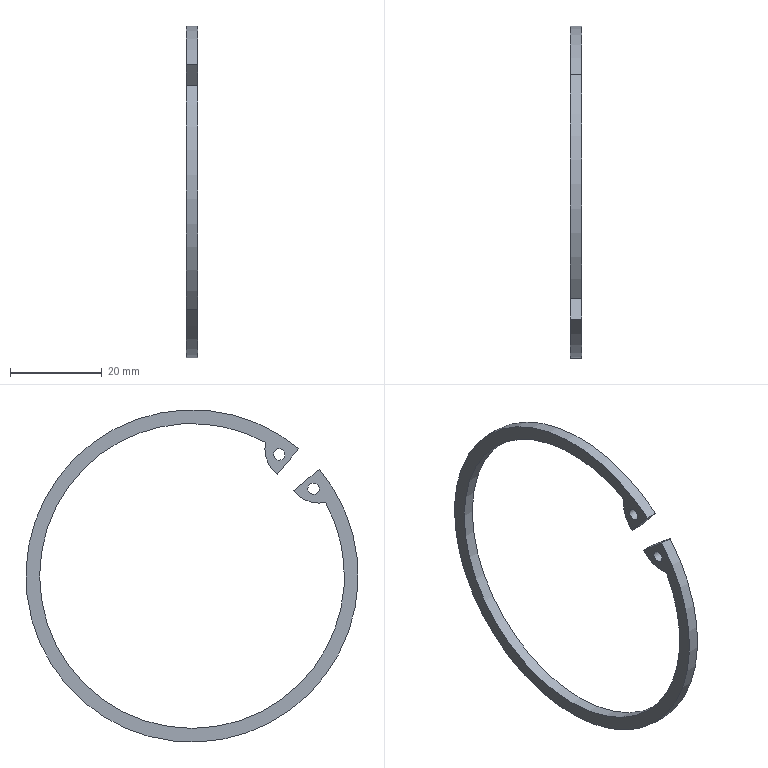Part | NX | features 4 2 | 1 solid | 16 faces | box 2.5 x 72.5 x 72.5 mm | volume 1667 mm3 | cylinder 12 | plane 4 | commonest cylinder face diameters 2.5 x4 66.5 x3 72.5 x3 14.8 x2
STEP:
#1=CARTESIAN_POINT('',(-160.5,-146.404,-801.98));
#2=VERTEX_POINT('',#1);
#3=CARTESIAN_POINT('',(-158.,-146.404,-801.98));
#4=VERTEX_POINT('',#3);
#5=CARTESIAN_POINT('',(-160.5,-146.404,-801.98));
#6=DIRECTION('',(1.,0.,0.));
#7=VECTOR('',#6,1000.);
#8=LINE('',#5,#7);
#9=EDGE_CURVE('',#2,#4,#8,.T.);
#10=ORIENTED_EDGE('',*,*,#9,.F.);
#11=CARTESIAN_POINT('',(-160.5,-144.636,-800.212));
#12=VERTEX_POINT('',#11);
#13=CARTESIAN_POINT('',(-160.5,-145.52,-801.096));
#14=DIRECTION('',(1.,0.,0.));
#15=DIRECTION('',(0.,0.7071,0.7071));
#16=AXIS2_PLACEMENT_3D('',#13,#14,#15);
#17=CIRCLE('',#16,1.25);
#18=EDGE_CURVE('',#12,#2,#17,.T.);
#19=ORIENTED_EDGE('',*,*,#18,.F.);
#20=CARTESIAN_POINT('',(-158.,-144.636,-800.212));
#21=VERTEX_POINT('',#20);
#22=CARTESIAN_POINT('',(-160.5,-144.636,-800.212));
#23=DIRECTION('',(1.,0.,0.));
#24=VECTOR('',#23,1000.);
#25=LINE('',#22,#24);
#26=EDGE_CURVE('',#21,#12,#25,.F.);
#27=ORIENTED_EDGE('',*,*,#26,.F.);
#28=CARTESIAN_POINT('',(-158.,-145.52,-801.096));
#29=DIRECTION('',(-1.,0.,0.));
#30=DIRECTION('',(0.,-0.7071,-0.7071));
#31=AXIS2_PLACEMENT_3D('',#28,#29,#30);
#32=CIRCLE('',#31,1.25);
#33=EDGE_CURVE('',#4,#21,#32,.T.);
#34=ORIENTED_EDGE('',*,*,#33,.F.);
#35=EDGE_LOOP('',(#10,#19,#27,#34));
#36=FACE_BOUND('',#35,.T.);
#37=CARTESIAN_POINT('',(-160.5,-145.52,-801.096));
#38=DIRECTION('',(-1.,0.,0.));
#39=DIRECTION('',(0.,0.7071,0.7071));
#40=AXIS2_PLACEMENT_3D('',#37,#38,#39);
#41=CYLINDRICAL_SURFACE('',#40,1.25);
#42=ADVANCED_FACE('',(#36),#41,.F.);
#43=CARTESIAN_POINT('',(-158.,-145.52,-801.096));
#44=DIRECTION('',(-1.,0.,0.));
#45=DIRECTION('',(0.,0.7071,0.7071));
#46=AXIS2_PLACEMENT_3D('',#43,#44,#45);
#47=CIRCLE('',#46,1.25);
#48=EDGE_CURVE('',#21,#4,#47,.T.);
#49=ORIENTED_EDGE('',*,*,#48,.F.);
#50=ORIENTED_EDGE('',*,*,#26,.T.);
#51=CARTESIAN_POINT('',(-160.5,-145.52,-801.096));
#52=DIRECTION('',(1.,0.,0.));
#53=DIRECTION('',(0.,-0.7071,-0.7071));
#54=AXIS2_PLACEMENT_3D('',#51,#52,#53);
#55=CIRCLE('',#54,1.25);
#56=EDGE_CURVE('',#2,#12,#55,.T.);
#57=ORIENTED_EDGE('',*,*,#56,.F.);
#58=ORIENTED_EDGE('',*,*,#9,.T.);
#59=EDGE_LOOP('',(#49,#50,#57,#58));
#60=FACE_BOUND('',#59,.T.);
#61=CARTESIAN_POINT('',(-160.5,-145.52,-801.096));
#62=DIRECTION('',(-1.,0.,0.));
#63=DIRECTION('',(0.,0.7071,0.7071));
#64=AXIS2_PLACEMENT_3D('',#61,#62,#63);
#65=CYLINDRICAL_SURFACE('',#64,1.25);
#66=ADVANCED_FACE('',(#60),#65,.F.);
#67=CARTESIAN_POINT('',(-158.,-137.149,-792.725));
#68=VERTEX_POINT('',#67);
#69=CARTESIAN_POINT('',(-158.,-138.917,-794.493));
#70=VERTEX_POINT('',#69);
#71=CARTESIAN_POINT('',(-158.,-138.033,-793.609));
#72=DIRECTION('',(-1.,0.,0.));
#73=DIRECTION('',(0.,0.7071,0.7071));
#74=AXIS2_PLACEMENT_3D('',#71,#72,#73);
#75=CIRCLE('',#74,1.25);
#76=EDGE_CURVE('',#68,#70,#75,.T.);
#77=ORIENTED_EDGE('',*,*,#76,.F.);
#78=CARTESIAN_POINT('',(-160.5,-137.149,-792.725));
#79=VERTEX_POINT('',#78);
#80=CARTESIAN_POINT('',(-160.5,-137.149,-792.725));
#81=DIRECTION('',(1.,0.,0.));
#82=VECTOR('',#81,1000.);
#83=LINE('',#80,#82);
#84=EDGE_CURVE('',#79,#68,#83,.T.);
#85=ORIENTED_EDGE('',*,*,#84,.F.);
#86=CARTESIAN_POINT('',(-160.5,-138.917,-794.493));
#87=VERTEX_POINT('',#86);
#88=CARTESIAN_POINT('',(-160.5,-138.033,-793.609));
#89=DIRECTION('',(1.,0.,0.));
#90=DIRECTION('',(0.,-0.7071,-0.7071));
#91=AXIS2_PLACEMENT_3D('',#88,#89,#90);
#92=CIRCLE('',#91,1.25);
#93=EDGE_CURVE('',#87,#79,#92,.T.);
#94=ORIENTED_EDGE('',*,*,#93,.F.);
#95=CARTESIAN_POINT('',(-160.5,-138.917,-794.493));
#96=DIRECTION('',(1.,0.,0.));
#97=VECTOR('',#96,1000.);
#98=LINE('',#95,#97);
#99=EDGE_CURVE('',#70,#87,#98,.F.);
#100=ORIENTED_EDGE('',*,*,#99,.F.);
#101=EDGE_LOOP('',(#77,#85,#94,#100));
#102=FACE_BOUND('',#101,.T.);
#103=CARTESIAN_POINT('',(-160.5,-138.033,-793.609));
#104=DIRECTION('',(-1.,0.,0.));
#105=DIRECTION('',(0.,0.7071,0.7071));
#106=AXIS2_PLACEMENT_3D('',#103,#104,#105);
#107=CYLINDRICAL_SURFACE('',#106,1.25);
#108=ADVANCED_FACE('',(#102),#107,.F.);
#109=CARTESIAN_POINT('',(-158.,-135.028,-790.997));
#110=VERTEX_POINT('',#109);
#111=CARTESIAN_POINT('',(-160.5,-135.028,-790.997));
#112=VERTEX_POINT('',#111);
#113=CARTESIAN_POINT('',(-158.,-135.028,-790.997));
#114=DIRECTION('',(-1.,0.,0.));
#115=VECTOR('',#114,1000.);
#116=LINE('',#113,#115);
#117=EDGE_CURVE('',#110,#112,#116,.T.);
#118=ORIENTED_EDGE('',*,*,#117,.F.);
#119=CARTESIAN_POINT('',(-158.,-137.544,-798.029));
#120=VERTEX_POINT('',#119);
#121=CARTESIAN_POINT('',(-158.,-142.301,-792.36));
#122=DIRECTION('',(1.,0.,0.));
#123=DIRECTION('',(0.,0.6428,-0.766));
#124=AXIS2_PLACEMENT_3D('',#121,#122,#123);
#125=CIRCLE('',#124,7.4);
#126=EDGE_CURVE('',#120,#110,#125,.T.);
#127=ORIENTED_EDGE('',*,*,#126,.F.);
#128=CARTESIAN_POINT('',(-160.5,-137.544,-798.029));
#129=VERTEX_POINT('',#128);
#130=CARTESIAN_POINT('',(-158.,-137.544,-798.029));
#131=DIRECTION('',(-1.,0.,0.));
#132=VECTOR('',#131,1000.);
#133=LINE('',#130,#132);
#134=EDGE_CURVE('',#120,#129,#133,.T.);
#135=ORIENTED_EDGE('',*,*,#134,.T.);
#136=CARTESIAN_POINT('',(-160.5,-142.301,-792.36));
#137=DIRECTION('',(-1.,0.,0.));
#138=DIRECTION('',(0.,0.9829,0.1842));
#139=AXIS2_PLACEMENT_3D('',#136,#137,#138);
#140=CIRCLE('',#139,7.4);
#141=EDGE_CURVE('',#112,#129,#140,.T.);
#142=ORIENTED_EDGE('',*,*,#141,.F.);
#143=EDGE_LOOP('',(#118,#127,#135,#142));
#144=FACE_BOUND('',#143,.T.);
#145=CARTESIAN_POINT('',(-160.5,-142.301,-792.36));
#146=DIRECTION('',(-1.,0.,0.));
#147=DIRECTION('',(0.,0.7071,0.7071));
#148=AXIS2_PLACEMENT_3D('',#145,#146,#147);
#149=CYLINDRICAL_SURFACE('',#148,7.4);
#150=ADVANCED_FACE('',(#144),#149,.T.);
#151=ORIENTED_EDGE('',*,*,#134,.F.);
#152=CARTESIAN_POINT('',(-158.,-142.301,-792.36));
#153=VERTEX_POINT('',#152);
#154=CARTESIAN_POINT('',(-158.,-142.301,-792.36));
#155=DIRECTION('',(0.,0.6428,-0.766));
#156=VECTOR('',#155,1000.);
#157=LINE('',#154,#156);
#158=EDGE_CURVE('',#153,#120,#157,.T.);
#159=ORIENTED_EDGE('',*,*,#158,.F.);
#160=CARTESIAN_POINT('',(-160.5,-142.301,-792.36));
#161=VERTEX_POINT('',#160);
#162=CARTESIAN_POINT('',(-160.5,-142.301,-792.36));
#163=DIRECTION('',(1.,0.,0.));
#164=VECTOR('',#163,1000.);
#165=LINE('',#162,#164);
#166=EDGE_CURVE('',#161,#153,#165,.T.);
#167=ORIENTED_EDGE('',*,*,#166,.F.);
#168=CARTESIAN_POINT('',(-160.5,-137.544,-798.029));
#169=DIRECTION('',(0.,-0.6428,0.766));
#170=VECTOR('',#169,1000.);
#171=LINE('',#168,#170);
#172=EDGE_CURVE('',#129,#161,#171,.T.);
#173=ORIENTED_EDGE('',*,*,#172,.F.);
#174=EDGE_LOOP('',(#151,#159,#167,#173));
#175=FACE_BOUND('',#174,.T.);
#176=CARTESIAN_POINT('',(-160.5,-137.544,-798.029));
#177=DIRECTION('',(0.,-0.766,-0.6428));
#178=DIRECTION('',(0.,0.6428,-0.766));
#179=AXIS2_PLACEMENT_3D('',#176,#177,#178);
#180=PLANE('',#179);
#181=ADVANCED_FACE('',(#175),#180,.T.);
#182=CARTESIAN_POINT('',(-160.5,-93.367,-794.497));
#183=VERTEX_POINT('',#182);
#184=CARTESIAN_POINT('',(-158.,-93.367,-794.497));
#185=VERTEX_POINT('',#184);
#186=CARTESIAN_POINT('',(-160.5,-93.367,-794.497));
#187=DIRECTION('',(1.,0.,0.));
#188=VECTOR('',#187,1000.);
#189=LINE('',#186,#188);
#190=EDGE_CURVE('',#183,#185,#189,.T.);
#191=ORIENTED_EDGE('',*,*,#190,.F.);
#192=CARTESIAN_POINT('',(-160.5,-119.,-820.129));
#193=DIRECTION('',(-1.,0.,0.));
#194=DIRECTION('',(0.,-0.6428,0.766));
#195=AXIS2_PLACEMENT_3D('',#192,#193,#194);
#196=CIRCLE('',#195,36.25);
#197=EDGE_CURVE('',#161,#183,#196,.T.);
#198=ORIENTED_EDGE('',*,*,#197,.F.);
#199=ORIENTED_EDGE('',*,*,#166,.T.);
#200=CARTESIAN_POINT('',(-158.,-119.,-820.129));
#201=DIRECTION('',(1.,0.,0.));
#202=DIRECTION('',(0.,0.7071,0.7071));
#203=AXIS2_PLACEMENT_3D('',#200,#201,#202);
#204=CIRCLE('',#203,36.25);
#205=EDGE_CURVE('',#185,#153,#204,.T.);
#206=ORIENTED_EDGE('',*,*,#205,.F.);
#207=EDGE_LOOP('',(#191,#198,#199,#206));
#208=FACE_BOUND('',#207,.T.);
#209=CARTESIAN_POINT('',(-160.5,-119.,-820.129));
#210=DIRECTION('',(-1.,0.,0.));
#211=DIRECTION('',(0.,0.7071,0.7071));
#212=AXIS2_PLACEMENT_3D('',#209,#210,#211);
#213=CYLINDRICAL_SURFACE('',#212,36.25);
#214=ADVANCED_FACE('',(#208),#213,.T.);
#215=CARTESIAN_POINT('',(-160.5,-144.633,-845.762));
#216=VERTEX_POINT('',#215);
#217=CARTESIAN_POINT('',(-158.,-144.633,-845.762));
#218=VERTEX_POINT('',#217);
#219=CARTESIAN_POINT('',(-160.5,-144.633,-845.762));
#220=DIRECTION('',(1.,0.,0.));
#221=VECTOR('',#220,1000.);
#222=LINE('',#219,#221);
#223=EDGE_CURVE('',#216,#218,#222,.T.);
#224=ORIENTED_EDGE('',*,*,#223,.F.);
#225=CARTESIAN_POINT('',(-160.5,-119.,-820.129));
#226=DIRECTION('',(-1.,0.,0.));
#227=DIRECTION('',(0.,0.7071,0.7071));
#228=AXIS2_PLACEMENT_3D('',#225,#226,#227);
#229=CIRCLE('',#228,36.25);
#230=EDGE_CURVE('',#183,#216,#229,.T.);
#231=ORIENTED_EDGE('',*,*,#230,.F.);
#232=ORIENTED_EDGE('',*,*,#190,.T.);
#233=CARTESIAN_POINT('',(-158.,-119.,-820.129));
#234=DIRECTION('',(1.,0.,0.));
#235=DIRECTION('',(0.,-0.7071,-0.7071));
#236=AXIS2_PLACEMENT_3D('',#233,#234,#235);
#237=CIRCLE('',#236,36.25);
#238=EDGE_CURVE('',#218,#185,#237,.T.);
#239=ORIENTED_EDGE('',*,*,#238,.F.);
#240=EDGE_LOOP('',(#224,#231,#232,#239));
#241=FACE_BOUND('',#240,.T.);
#242=CARTESIAN_POINT('',(-160.5,-119.,-820.129));
#243=DIRECTION('',(-1.,0.,0.));
#244=DIRECTION('',(0.,0.7071,0.7071));
#245=AXIS2_PLACEMENT_3D('',#242,#243,#244);
#246=CYLINDRICAL_SURFACE('',#245,36.25);
#247=ADVANCED_FACE('',(#241),#246,.T.);
#248=CARTESIAN_POINT('',(-158.,-146.769,-796.828));
#249=VERTEX_POINT('',#248);
#250=CARTESIAN_POINT('',(-158.,-119.,-820.129));
#251=DIRECTION('',(1.,0.,0.));
#252=DIRECTION('',(0.,-0.766,0.6428));
#253=AXIS2_PLACEMENT_3D('',#250,#251,#252);
#254=CIRCLE('',#253,36.25);
#255=EDGE_CURVE('',#249,#218,#254,.T.);
#256=ORIENTED_EDGE('',*,*,#255,.F.);
#257=CARTESIAN_POINT('',(-160.5,-146.769,-796.828));
#258=VERTEX_POINT('',#257);
#259=CARTESIAN_POINT('',(-158.,-146.769,-796.828));
#260=DIRECTION('',(-1.,0.,0.));
#261=VECTOR('',#260,1000.);
#262=LINE('',#259,#261);
#263=EDGE_CURVE('',#249,#258,#262,.T.);
#264=ORIENTED_EDGE('',*,*,#263,.T.);
#265=CARTESIAN_POINT('',(-160.5,-119.,-820.129));
#266=DIRECTION('',(-1.,0.,0.));
#267=DIRECTION('',(0.,-0.7071,-0.7071));
#268=AXIS2_PLACEMENT_3D('',#265,#266,#267);
#269=CIRCLE('',#268,36.25);
#270=EDGE_CURVE('',#216,#258,#269,.T.);
#271=ORIENTED_EDGE('',*,*,#270,.F.);
#272=ORIENTED_EDGE('',*,*,#223,.T.);
#273=EDGE_LOOP('',(#256,#264,#271,#272));
#274=FACE_BOUND('',#273,.T.);
#275=CARTESIAN_POINT('',(-160.5,-119.,-820.129));
#276=DIRECTION('',(-1.,0.,0.));
#277=DIRECTION('',(0.,0.7071,0.7071));
#278=AXIS2_PLACEMENT_3D('',#275,#276,#277);
#279=CYLINDRICAL_SURFACE('',#278,36.25);
#280=ADVANCED_FACE('',(#274),#279,.T.);
#281=ORIENTED_EDGE('',*,*,#263,.F.);
#282=CARTESIAN_POINT('',(-158.,-141.1,-801.585));
#283=VERTEX_POINT('',#282);
#284=CARTESIAN_POINT('',(-158.,-141.1,-801.585));
#285=DIRECTION('',(0.,-0.766,0.6428));
#286=VECTOR('',#285,1000.);
#287=LINE('',#284,#286);
#288=EDGE_CURVE('',#283,#249,#287,.T.);
#289=ORIENTED_EDGE('',*,*,#288,.F.);
#290=CARTESIAN_POINT('',(-160.5,-141.1,-801.585));
#291=VERTEX_POINT('',#290);
#292=CARTESIAN_POINT('',(-160.5,-141.1,-801.585));
#293=DIRECTION('',(1.,0.,0.));
#294=VECTOR('',#293,1000.);
#295=LINE('',#292,#294);
#296=EDGE_CURVE('',#291,#283,#295,.T.);
#297=ORIENTED_EDGE('',*,*,#296,.F.);
#298=CARTESIAN_POINT('',(-160.5,-146.769,-796.828));
#299=DIRECTION('',(0.,0.766,-0.6428));
#300=VECTOR('',#299,1000.);
#301=LINE('',#298,#300);
#302=EDGE_CURVE('',#258,#291,#301,.T.);
#303=ORIENTED_EDGE('',*,*,#302,.F.);
#304=EDGE_LOOP('',(#281,#289,#297,#303));
#305=FACE_BOUND('',#304,.T.);
#306=CARTESIAN_POINT('',(-160.5,-146.769,-796.828));
#307=DIRECTION('',(0.,0.6428,0.766));
#308=DIRECTION('',(0.,-0.766,0.6428));
#309=AXIS2_PLACEMENT_3D('',#306,#307,#308);
#310=PLANE('',#309);
#311=ADVANCED_FACE('',(#305),#310,.T.);
#312=ORIENTED_EDGE('',*,*,#18,.T.);
#313=ORIENTED_EDGE('',*,*,#56,.T.);
#314=EDGE_LOOP('',(#312,#313));
#315=FACE_BOUND('',#314,.T.);
#316=CARTESIAN_POINT('',(-160.5,-138.033,-793.609));
#317=DIRECTION('',(1.,0.,0.));
#318=DIRECTION('',(0.,0.7071,0.7071));
#319=AXIS2_PLACEMENT_3D('',#316,#317,#318);
#320=CIRCLE('',#319,1.25);
#321=EDGE_CURVE('',#79,#87,#320,.T.);
#322=ORIENTED_EDGE('',*,*,#321,.T.);
#323=ORIENTED_EDGE('',*,*,#93,.T.);
#324=EDGE_LOOP('',(#322,#323));
#325=FACE_BOUND('',#324,.T.);
#326=CARTESIAN_POINT('',(-160.5,-148.132,-804.102));
#327=VERTEX_POINT('',#326);
#328=CARTESIAN_POINT('',(-160.5,-146.769,-796.828));
#329=DIRECTION('',(-1.,0.,0.));
#330=DIRECTION('',(0.,0.766,-0.6428));
#331=AXIS2_PLACEMENT_3D('',#328,#329,#330);
#332=CIRCLE('',#331,7.4);
#333=EDGE_CURVE('',#291,#327,#332,.T.);
#334=ORIENTED_EDGE('',*,*,#333,.T.);
#335=CARTESIAN_POINT('',(-160.5,-142.511,-843.641));
#336=VERTEX_POINT('',#335);
#337=CARTESIAN_POINT('',(-160.5,-119.,-820.129));
#338=DIRECTION('',(1.,0.,0.));
#339=DIRECTION('',(0.,-0.8762,0.482));
#340=AXIS2_PLACEMENT_3D('',#337,#338,#339);
#341=CIRCLE('',#340,33.25);
#342=EDGE_CURVE('',#327,#336,#341,.T.);
#343=ORIENTED_EDGE('',*,*,#342,.T.);
#344=CARTESIAN_POINT('',(-160.5,-95.489,-796.618));
#345=VERTEX_POINT('',#344);
#346=CARTESIAN_POINT('',(-160.5,-119.,-820.129));
#347=DIRECTION('',(1.,0.,0.));
#348=DIRECTION('',(0.,-0.7071,-0.7071));
#349=AXIS2_PLACEMENT_3D('',#346,#347,#348);
#350=CIRCLE('',#349,33.25);
#351=EDGE_CURVE('',#336,#345,#350,.T.);
#352=ORIENTED_EDGE('',*,*,#351,.T.);
#353=CARTESIAN_POINT('',(-160.5,-119.,-820.129));
#354=DIRECTION('',(1.,0.,0.));
#355=DIRECTION('',(0.,0.7071,0.7071));
#356=AXIS2_PLACEMENT_3D('',#353,#354,#355);
#357=CIRCLE('',#356,33.25);
#358=EDGE_CURVE('',#345,#112,#357,.T.);
#359=ORIENTED_EDGE('',*,*,#358,.T.);
#360=ORIENTED_EDGE('',*,*,#141,.T.);
#361=ORIENTED_EDGE('',*,*,#172,.T.);
#362=ORIENTED_EDGE('',*,*,#197,.T.);
#363=ORIENTED_EDGE('',*,*,#230,.T.);
#364=ORIENTED_EDGE('',*,*,#270,.T.);
#365=ORIENTED_EDGE('',*,*,#302,.T.);
#366=EDGE_LOOP('',(#334,#343,#352,#359,#360,#361,#362,#363,#364,#365));
#367=FACE_BOUND('',#366,.T.);
#368=CARTESIAN_POINT('',(-160.5,-119.,-820.129));
#369=DIRECTION('',(1.,0.,0.));
#370=DIRECTION('',(0.,-0.7071,-0.7071));
#371=AXIS2_PLACEMENT_3D('',#368,#369,#370);
#372=PLANE('',#371);
#373=ADVANCED_FACE('',(#315,#325,#367),#372,.F.);
#374=ORIENTED_EDGE('',*,*,#296,.T.);
#375=CARTESIAN_POINT('',(-158.,-148.132,-804.102));
#376=VERTEX_POINT('',#375);
#377=CARTESIAN_POINT('',(-158.,-146.769,-796.828));
#378=DIRECTION('',(1.,0.,0.));
#379=DIRECTION('',(0.,-0.1842,-0.9829));
#380=AXIS2_PLACEMENT_3D('',#377,#378,#379);
#381=CIRCLE('',#380,7.4);
#382=EDGE_CURVE('',#376,#283,#381,.T.);
#383=ORIENTED_EDGE('',*,*,#382,.F.);
#384=CARTESIAN_POINT('',(-160.5,-148.132,-804.102));
#385=DIRECTION('',(1.,0.,0.));
#386=VECTOR('',#385,1000.);
#387=LINE('',#384,#386);
#388=EDGE_CURVE('',#327,#376,#387,.T.);
#389=ORIENTED_EDGE('',*,*,#388,.F.);
#390=ORIENTED_EDGE('',*,*,#333,.F.);
#391=EDGE_LOOP('',(#374,#383,#389,#390));
#392=FACE_BOUND('',#391,.T.);
#393=CARTESIAN_POINT('',(-160.5,-146.769,-796.828));
#394=DIRECTION('',(-1.,0.,0.));
#395=DIRECTION('',(0.,0.7071,0.7071));
#396=AXIS2_PLACEMENT_3D('',#393,#394,#395);
#397=CYLINDRICAL_SURFACE('',#396,7.4);
#398=ADVANCED_FACE('',(#392),#397,.T.);
#399=CARTESIAN_POINT('',(-158.,-142.511,-843.641));
#400=VERTEX_POINT('',#399);
#401=CARTESIAN_POINT('',(-160.5,-142.511,-843.641));
#402=DIRECTION('',(1.,0.,0.));
#403=VECTOR('',#402,1000.);
#404=LINE('',#401,#403);
#405=EDGE_CURVE('',#336,#400,#404,.T.);
#406=ORIENTED_EDGE('',*,*,#405,.F.);
#407=ORIENTED_EDGE('',*,*,#342,.F.);
#408=ORIENTED_EDGE('',*,*,#388,.T.);
#409=CARTESIAN_POINT('',(-158.,-119.,-820.129));
#410=DIRECTION('',(-1.,0.,0.));
#411=DIRECTION('',(0.,-0.7071,-0.7071));
#412=AXIS2_PLACEMENT_3D('',#409,#410,#411);
#413=CIRCLE('',#412,33.25);
#414=EDGE_CURVE('',#400,#376,#413,.T.);
#415=ORIENTED_EDGE('',*,*,#414,.F.);
#416=EDGE_LOOP('',(#406,#407,#408,#415));
#417=FACE_BOUND('',#416,.T.);
#418=CARTESIAN_POINT('',(-160.5,-119.,-820.129));
#419=DIRECTION('',(-1.,0.,0.));
#420=DIRECTION('',(0.,0.7071,0.7071));
#421=AXIS2_PLACEMENT_3D('',#418,#419,#420);
#422=CYLINDRICAL_SURFACE('',#421,33.25);
#423=ADVANCED_FACE('',(#417),#422,.F.);
#424=CARTESIAN_POINT('',(-158.,-95.489,-796.618));
#425=VERTEX_POINT('',#424);
#426=CARTESIAN_POINT('',(-158.,-119.,-820.129));
#427=DIRECTION('',(-1.,0.,0.));
#428=DIRECTION('',(0.,0.7071,0.7071));
#429=AXIS2_PLACEMENT_3D('',#426,#427,#428);
#430=CIRCLE('',#429,33.25);
#431=EDGE_CURVE('',#425,#400,#430,.T.);
#432=ORIENTED_EDGE('',*,*,#431,.F.);
#433=CARTESIAN_POINT('',(-160.5,-95.489,-796.618));
#434=DIRECTION('',(1.,0.,0.));
#435=VECTOR('',#434,1000.);
#436=LINE('',#433,#435);
#437=EDGE_CURVE('',#345,#425,#436,.T.);
#438=ORIENTED_EDGE('',*,*,#437,.F.);
#439=ORIENTED_EDGE('',*,*,#351,.F.);
#440=ORIENTED_EDGE('',*,*,#405,.T.);
#441=EDGE_LOOP('',(#432,#438,#439,#440));
#442=FACE_BOUND('',#441,.T.);
#443=CARTESIAN_POINT('',(-160.5,-119.,-820.129));
#444=DIRECTION('',(-1.,0.,0.));
#445=DIRECTION('',(0.,0.7071,0.7071));
#446=AXIS2_PLACEMENT_3D('',#443,#444,#445);
#447=CYLINDRICAL_SURFACE('',#446,33.25);
#448=ADVANCED_FACE('',(#442),#447,.F.);
#449=CARTESIAN_POINT('',(-158.,-119.,-820.129));
#450=DIRECTION('',(-1.,0.,0.));
#451=DIRECTION('',(0.,-0.482,0.8762));
#452=AXIS2_PLACEMENT_3D('',#449,#450,#451);
#453=CIRCLE('',#452,33.25);
#454=EDGE_CURVE('',#110,#425,#453,.T.);
#455=ORIENTED_EDGE('',*,*,#454,.F.);
#456=ORIENTED_EDGE('',*,*,#117,.T.);
#457=ORIENTED_EDGE('',*,*,#358,.F.);
#458=ORIENTED_EDGE('',*,*,#437,.T.);
#459=EDGE_LOOP('',(#455,#456,#457,#458));
#460=FACE_BOUND('',#459,.T.);
#461=CARTESIAN_POINT('',(-160.5,-119.,-820.129));
#462=DIRECTION('',(-1.,0.,0.));
#463=DIRECTION('',(0.,0.7071,0.7071));
#464=AXIS2_PLACEMENT_3D('',#461,#462,#463);
#465=CYLINDRICAL_SURFACE('',#464,33.25);
#466=ADVANCED_FACE('',(#460),#465,.F.);
#467=ORIENTED_EDGE('',*,*,#33,.T.);
#468=ORIENTED_EDGE('',*,*,#48,.T.);
#469=EDGE_LOOP('',(#467,#468));
#470=FACE_BOUND('',#469,.T.);
#471=CARTESIAN_POINT('',(-158.,-138.033,-793.609));
#472=DIRECTION('',(-1.,0.,0.));
#473=DIRECTION('',(0.,-0.7071,-0.7071));
#474=AXIS2_PLACEMENT_3D('',#471,#472,#473);
#475=CIRCLE('',#474,1.25);
#476=EDGE_CURVE('',#70,#68,#475,.T.);
#477=ORIENTED_EDGE('',*,*,#476,.T.);
#478=ORIENTED_EDGE('',*,*,#76,.T.);
#479=EDGE_LOOP('',(#477,#478));
#480=FACE_BOUND('',#479,.T.);
#481=ORIENTED_EDGE('',*,*,#431,.T.);
#482=ORIENTED_EDGE('',*,*,#414,.T.);
#483=ORIENTED_EDGE('',*,*,#382,.T.);
#484=ORIENTED_EDGE('',*,*,#288,.T.);
#485=ORIENTED_EDGE('',*,*,#255,.T.);
#486=ORIENTED_EDGE('',*,*,#238,.T.);
#487=ORIENTED_EDGE('',*,*,#205,.T.);
#488=ORIENTED_EDGE('',*,*,#158,.T.);
#489=ORIENTED_EDGE('',*,*,#126,.T.);
#490=ORIENTED_EDGE('',*,*,#454,.T.);
#491=EDGE_LOOP('',(#481,#482,#483,#484,#485,#486,#487,#488,#489,#490));
#492=FACE_BOUND('',#491,.T.);
#493=CARTESIAN_POINT('',(-158.,-119.,-820.129));
#494=DIRECTION('',(1.,0.,0.));
#495=DIRECTION('',(0.,-0.7071,-0.7071));
#496=AXIS2_PLACEMENT_3D('',#493,#494,#495);
#497=PLANE('',#496);
#498=ADVANCED_FACE('',(#470,#480,#492),#497,.T.);
#499=ORIENTED_EDGE('',*,*,#99,.T.);
#500=ORIENTED_EDGE('',*,*,#321,.F.);
#501=ORIENTED_EDGE('',*,*,#84,.T.);
#502=ORIENTED_EDGE('',*,*,#476,.F.);
#503=EDGE_LOOP('',(#499,#500,#501,#502));
#504=FACE_BOUND('',#503,.T.);
#505=CARTESIAN_POINT('',(-160.5,-138.033,-793.609));
#506=DIRECTION('',(-1.,0.,0.));
#507=DIRECTION('',(0.,0.7071,0.7071));
#508=AXIS2_PLACEMENT_3D('',#505,#506,#507);
#509=CYLINDRICAL_SURFACE('',#508,1.25);
#510=ADVANCED_FACE('',(#504),#509,.F.);
#511=CLOSED_SHELL('',(#42,#66,#108,#150,#181,#214,#247,#280,#311,#373,#398,#423,#448,#466,#498,#510));
#512=MANIFOLD_SOLID_BREP('',#511);
#513=(LENGTH_UNIT()NAMED_UNIT(*)SI_UNIT(.MILLI.,.METRE.));
#514=UNCERTAINTY_MEASURE_WITH_UNIT(LENGTH_MEASURE(0.00001),#513,'','');
#515=(NAMED_UNIT(*)PLANE_ANGLE_UNIT()SI_UNIT($,.RADIAN.));
#516=(NAMED_UNIT(*)SI_UNIT($,.STERADIAN.)SOLID_ANGLE_UNIT());
#517=(GEOMETRIC_REPRESENTATION_CONTEXT(3)GLOBAL_UNCERTAINTY_ASSIGNED_CONTEXT((#514))GLOBAL_UNIT_ASSIGNED_CONTEXT((#513,#515,#516))REPRESENTATION_CONTEXT('',''));
#518=ADVANCED_BREP_SHAPE_REPRESENTATION('',(#512),#517);